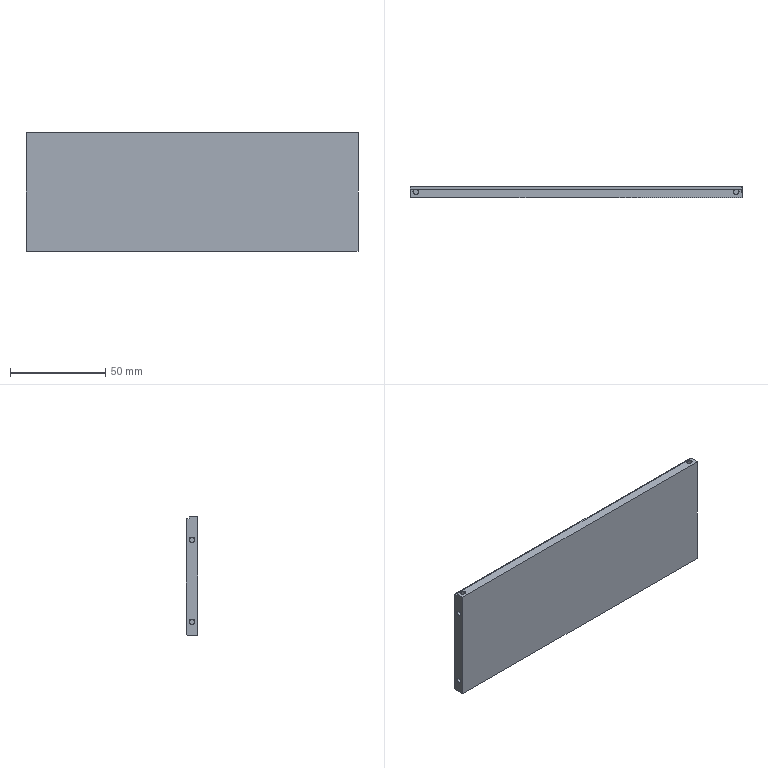Part | SolidWorks | features BaseBody 1 | 1 solid | 79 faces | box 174 x 6 x 62 mm | volume 63958 mm3 | cone 28 | cylinder 28 | plane 23 | commonest cylinder face diameters 3.5 x16 2.5 x12